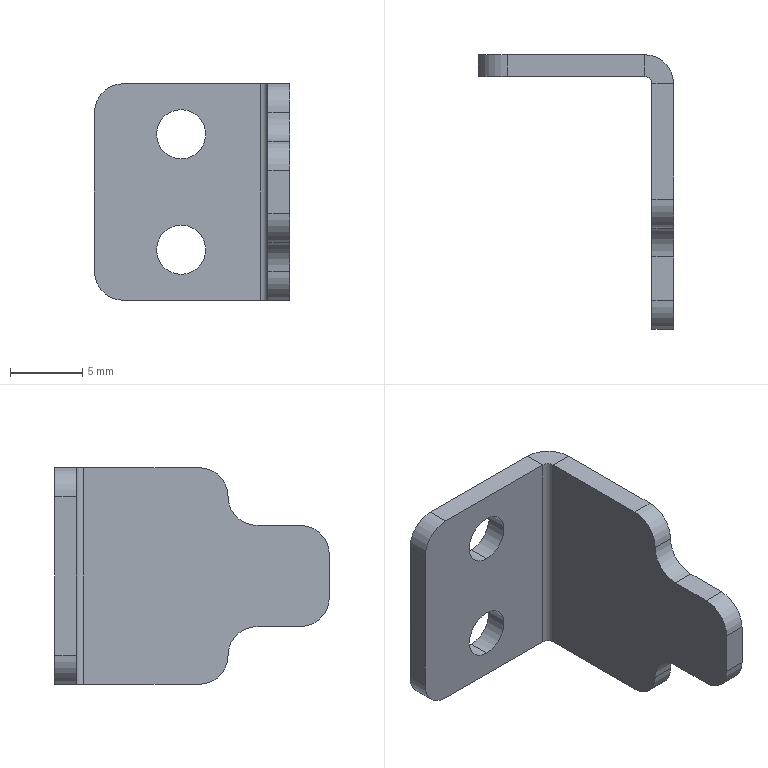Part | STEP file | 1 solid | 28 faces | box 13.5 x 19 x 15 mm | volume 569.041 mm3 | cylinder 14 | plane 14 | commonest cylinder face diameters 4 x9 3.4 x4 1 x1